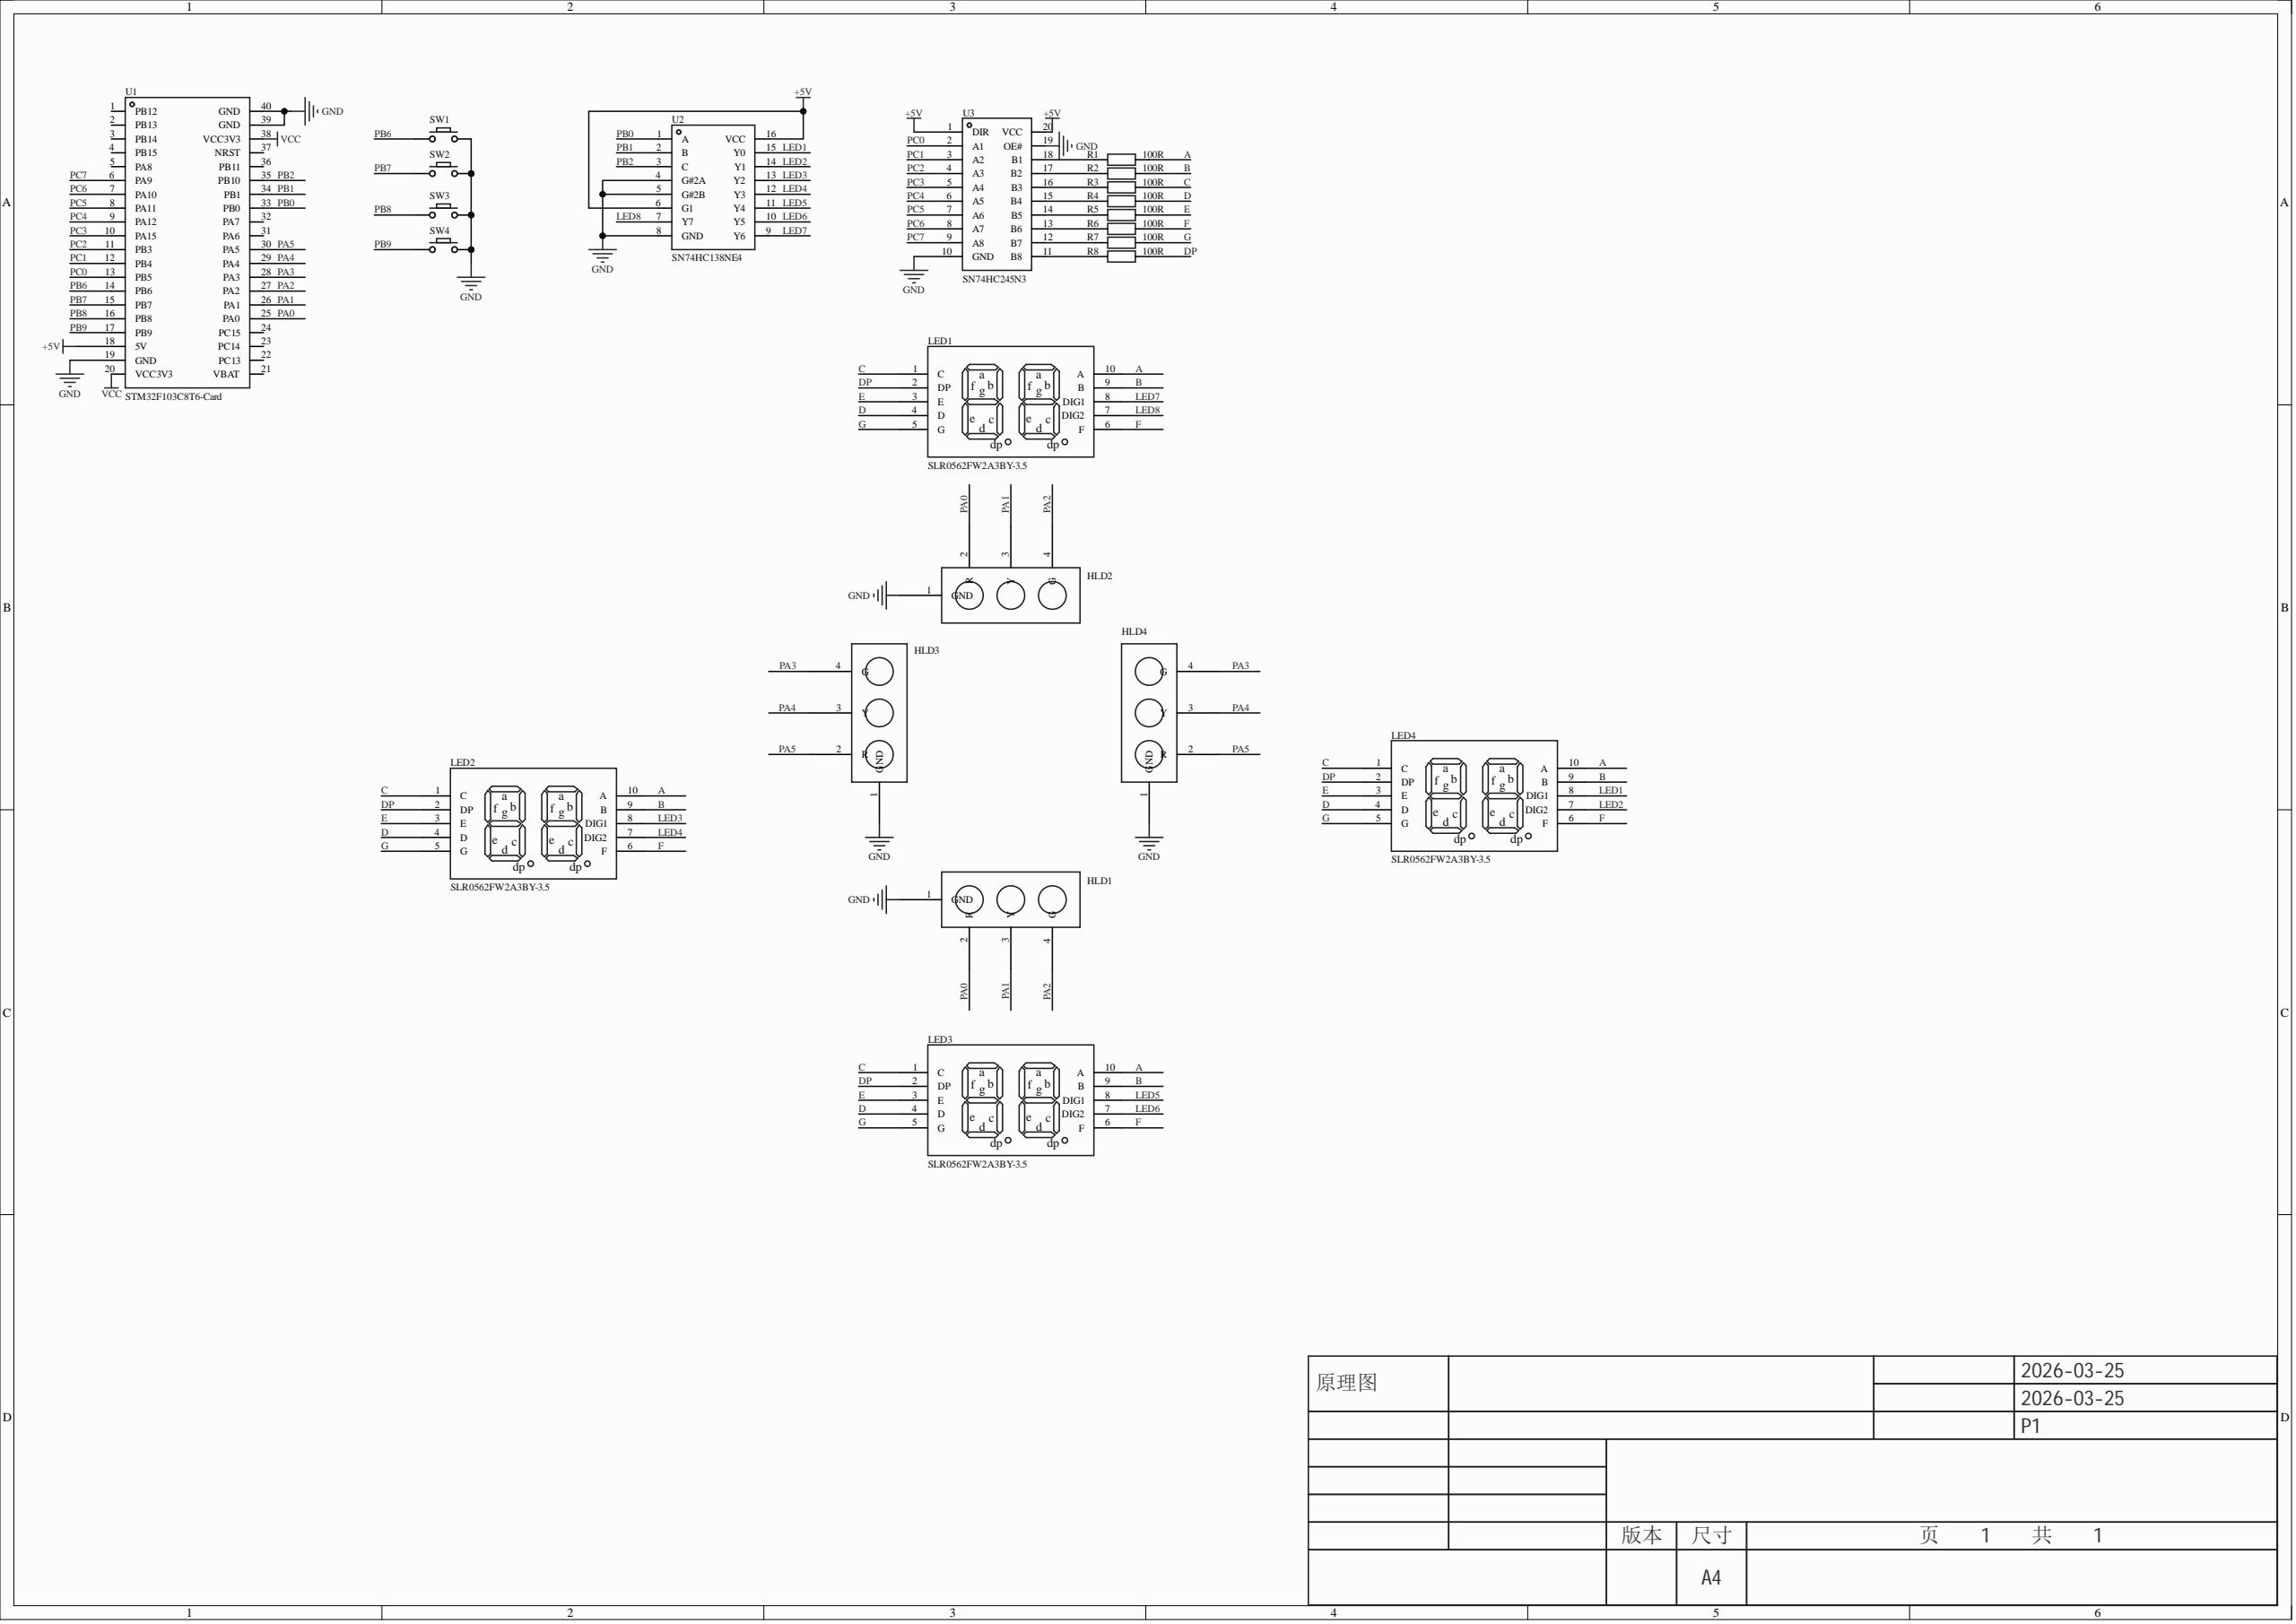Circuit board | Altium Designer | 23 parts | 48 nets
Bill of materials:
Comment,Description,Designator,Footprint,LibRef,Quantity
"","","HLD1, HLD2, HLD3, HLD4","SIP-04","RGY","4"
"SLR0562FW2A3BY-3.5","","LED1, LED2, LED3, LED4","LED-SEG-TH_10P-L25.0-W19.0-P2.54-S15.24-BL","SLR0562FW2A3BY-3.5","4"
"100R","","R1, R2, R3, R4, R5, R6, R7, R8","Res_1/8W","Res_AXIAL-1/8W","8"
"","","SW1, SW2, SW3, SW4","Key_TH_3.5x6x4.3","Key_TH_3.5x6x4.3","4"
"STM32F103C8T6-Card","","U1","CONN-TH_L53.3-W22.9_STM32F103C8T6-CARD","STM32F103C8T6-Card","1"
"SN74HC138NE4","","U2","PDIP-16_L19.7-W6.6-P2.54-LS7.6-BL","SN74HC138NE4","1"
"SN74HC245N3","","U3","PDIP-20_L25.9-W6.6-P2.54-LS7.9-BL","SN74HC245N3","1"
Netlist (Protel format):
[
HLD1
SIP-04




]
[
HLD2
SIP-04




]
[
HLD3
SIP-04




]
[
HLD4
SIP-04




]
[
LED1
LED-SEG-TH_10P-L25.0-W19.0-P2.54-S15.24-BL
SLR0562FW2A3BY-3.5



]
[
LED2
LED-SEG-TH_10P-L25.0-W19.0-P2.54-S15.24-BL
SLR0562FW2A3BY-3.5



]
[
LED3
LED-SEG-TH_10P-L25.0-W19.0-P2.54-S15.24-BL
SLR0562FW2A3BY-3.5



]
[
LED4
LED-SEG-TH_10P-L25.0-W19.0-P2.54-S15.24-BL
SLR0562FW2A3BY-3.5



]
[
R1
Res_1/8W
100R



]
[
R2
Res_1/8W
100R



]
[
R3
Res_1/8W
100R



]
[
R4
Res_1/8W
100R



]
[
R5
Res_1/8W
100R



]
[
R6
Res_1/8W
100R



]
[
R7
Res_1/8W
100R



]
[
R8
Res_1/8W
100R



]
[
SW1
Key_TH_3.5x6x4.3




]
[
SW2
Key_TH_3.5x6x4.3




]
[
SW3
Key_TH_3.5x6x4.3




]
[
SW4
Key_TH_3.5x6x4.3




]
[
U1
CONN-TH_L53.3-W22.9_STM32F103C8T6-CARD
STM32F103C8T6-Card



]
[
U2
PDIP-16_L19.7-W6.6-P2.54-LS7.6-BL
SN74HC138NE4



]
[
U3
PDIP-20_L25.9-W6.6-P2.54-LS7.9-BL
SN74HC245N3



]
(
VCC
U1-20
U1-38
)
(
PC7
U1-6
U3-9
)
(
PC6
U1-7
U3-8
)
(
PC5
U1-8
U3-7
)
(
PC4
U1-9
U3-6
)
(
PC3
U1-10
U3-5
)
(
PC2
U1-11
U3-4
)
(
PC1
U1-12
U3-3
)
(
PC0
U1-13
U3-2
)
(
PB9
SW4-A
U1-17
)
(
PB8
SW3-A
U1-16
)
(
PB7
SW2-A
U1-15
)
(
PB6
SW1-A
U1-14
)
(
PB2
U1-35
U2-3
)
(
PB1
U1-34
U2-2
)
(
PB0
U1-33
U2-1
)
(
PA5
HLD3-2
HLD4-2
U1-30
)
(
PA4
HLD3-3
HLD4-3
U1-29
)
(
PA3
HLD3-4
HLD4-4
U1-28
)
(
PA2
HLD1-4
HLD2-4
U1-27
)
(
PA1
HLD1-3
HLD2-3
U1-26
)
(
PA0
HLD1-2
HLD2-2
U1-25
)
(
NetR8_1
R8-1
U3-11
)
(
NetR7_1
R7-1
U3-12
)
(
NetR6_1
R6-1
U3-13
)
(
NetR5_1
R5-1
U3-14
)
(
NetR4_1
R4-1
U3-15
)
(
NetR3_1
R3-1
U3-16
)
(
NetR2_1
R2-1
U3-17
)
(
NetR1_1
R1-1
U3-18
)
(
LED8
LED1-7
U2-7
)
(
LED7
LED1-8
U2-9
)
(
LED6
LED3-7
U2-10
)
(
LED5
LED3-8
U2-11
)
(
LED4
LED2-7
U2-12
)
(
LED3
LED2-8
U2-13
)
(
LED2
LED4-7
U2-14
)
(
LED1
LED4-8
U2-15
)
(
GND
HLD1-1
HLD2-1
HLD3-1
HLD4-1
SW1-B
SW2-B
SW3-B
SW4-B
U1-19
U1-39
U1-40
U2-4
U2-5
U2-8
U3-10
U3-19
)
(
G
LED1-5
LED2-5
LED3-5
LED4-5
R7-2
)
(
F
LED1-6
LED2-6
LED3-6
LED4-6
R6-2
)
(
E
LED1-3
LED2-3
LED3-3
LED4-3
R5-2
)
(
DP
LED1-2
LED2-2
LED3-2
LED4-2
R8-2
)
(
D
LED1-4
LED2-4
LED3-4
LED4-4
R4-2
)
(
C
LED1-1
LED2-1
LED3-1
LED4-1
R3-2
)
(
B
LED1-9
LED2-9
LED3-9
LED4-9
R2-2
)
(
A
LED1-10
LED2-10
LED3-10
LED4-10
R1-2
)
(
+5V
U1-18
U2-6
U2-16
U3-1
U3-20
)